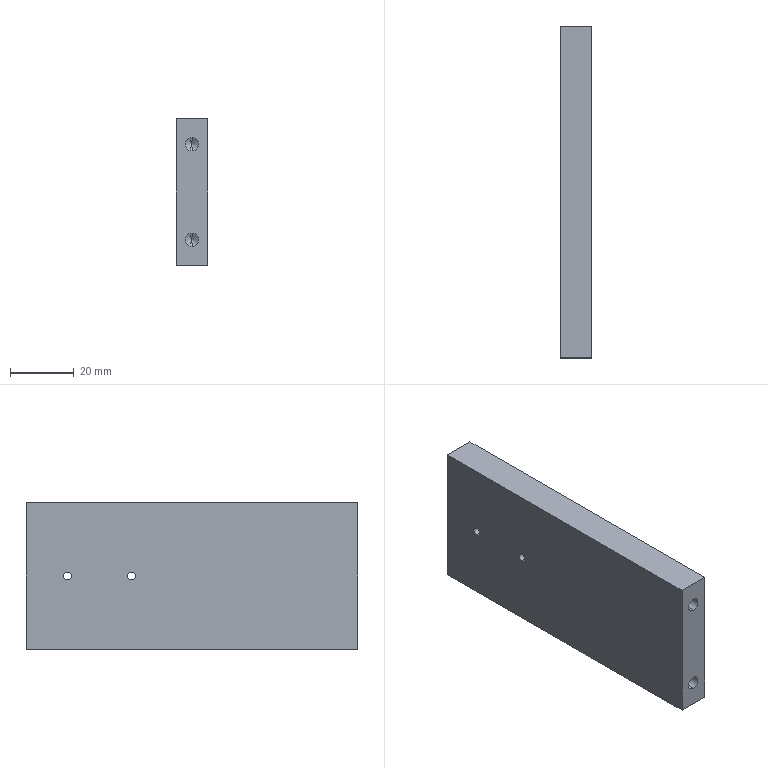Part | STEP file | 2058 Cylinder mounting plate | 1 solid | 18 faces | box 10 x 104 x 46 mm | volume 47342 mm3 | cylinder 8 | plane 6 | cone 4 | commonest cylinder face diameters 2.5 x4 4.2 x4
STEP:
#1=CARTESIAN_POINT('',(0.,0.,0.));
#2=DIRECTION('',(0.,0.,1.));
#3=DIRECTION('',(1.,0.,0.));
#4=AXIS2_PLACEMENT_3D('',#1,#2,#3);
#5=CARTESIAN_POINT('',(0.,-38.,5.9));
#6=VERTEX_POINT('',#5);
#7=CARTESIAN_POINT('',(0.,-52.,5.9));
#8=VERTEX_POINT('',#7);
#9=CARTESIAN_POINT('',(0.,-52.,5.9));
#10=DIRECTION('',(0.,-1.,0.));
#11=VECTOR('',#10,1.);
#12=LINE('',#9,#11);
#13=CARTESIAN_POINT('',(0.,-52.,8.));
#14=DIRECTION('',(0.,-1.,0.));
#15=DIRECTION('',(0.,0.,-1.));
#16=AXIS2_PLACEMENT_3D('',#13,#14,#15);
#17=CYLINDRICAL_SURFACE('',#16,2.1);
#18=CARTESIAN_POINT('',(6.283,0.));
#19=DIRECTION('',(0.,1.));
#20=VECTOR('',#19,1.);
#21=LINE('',#18,#20);
#22=(GEOMETRIC_REPRESENTATION_CONTEXT(2)PARAMETRIC_REPRESENTATION_CONTEXT()REPRESENTATION_CONTEXT('',''));
#23=DEFINITIONAL_REPRESENTATION('',(#21),#22);
#24=PCURVE('',#17,#23);
#25=CARTESIAN_POINT('',(0.,-52.,8.));
#26=DIRECTION('',(0.,-1.,0.));
#27=DIRECTION('',(0.,0.,-1.));
#28=AXIS2_PLACEMENT_3D('',#25,#26,#27);
#29=CYLINDRICAL_SURFACE('',#28,2.1);
#30=CARTESIAN_POINT('',(0.,0.));
#31=DIRECTION('',(0.,1.));
#32=VECTOR('',#31,1.);
#33=LINE('',#30,#32);
#34=(GEOMETRIC_REPRESENTATION_CONTEXT(2)PARAMETRIC_REPRESENTATION_CONTEXT()REPRESENTATION_CONTEXT('',''));
#35=DEFINITIONAL_REPRESENTATION('',(#33),#34);
#36=PCURVE('',#29,#35);
#37=SURFACE_CURVE('',#12,(#24,#36),.PCURVE_S1.);
#38=EDGE_CURVE('',#6,#8,#37,.T.);
#39=ORIENTED_EDGE('',*,*,#38,.T.);
#40=CARTESIAN_POINT('',(0.,-52.,10.1));
#41=VERTEX_POINT('',#40);
#42=CARTESIAN_POINT('',(0.,-52.,8.));
#43=DIRECTION('',(0.,-1.,0.));
#44=DIRECTION('',(0.,0.,-1.));
#45=AXIS2_PLACEMENT_3D('',#42,#43,#44);
#46=CIRCLE('',#45,2.1);
#47=CARTESIAN_POINT('',(0.,0.));
#48=DIRECTION('',(1.,0.));
#49=VECTOR('',#48,1.);
#50=LINE('',#47,#49);
#51=(GEOMETRIC_REPRESENTATION_CONTEXT(2)PARAMETRIC_REPRESENTATION_CONTEXT()REPRESENTATION_CONTEXT('',''));
#52=DEFINITIONAL_REPRESENTATION('',(#50),#51);
#53=PCURVE('',#17,#52);
#54=CARTESIAN_POINT('',(-5.,-52.,46.));
#55=DIRECTION('',(0.,1.,0.));
#56=DIRECTION('',(0.,0.,1.));
#57=AXIS2_PLACEMENT_3D('',#54,#55,#56);
#58=PLANE('',#57);
#59=CARTESIAN_POINT('',(-40.1,5.));
#60=CARTESIAN_POINT('',(-40.1,8.637));
#61=CARTESIAN_POINT('',(-36.95,6.819));
#62=CARTESIAN_POINT('',(-33.8,5.));
#63=CARTESIAN_POINT('',(-36.95,3.181));
#64=CARTESIAN_POINT('',(-40.1,1.363));
#65=CARTESIAN_POINT('',(-40.1,5.));
#66=(BOUNDED_CURVE()B_SPLINE_CURVE(2,(#59,#60,#61,#62,#63,#64,#65),.UNSPECIFIED.,.T.,.F.)B_SPLINE_CURVE_WITH_KNOTS((1,2,2,2,2,1),(-2.094,0.,2.094,4.189,6.283,8.378),.UNSPECIFIED.)CURVE()GEOMETRIC_REPRESENTATION_ITEM()RATIONAL_B_SPLINE_CURVE((1.,0.5,1.,0.5,1.,0.5,1.))REPRESENTATION_ITEM(''));
#67=(GEOMETRIC_REPRESENTATION_CONTEXT(2)PARAMETRIC_REPRESENTATION_CONTEXT()REPRESENTATION_CONTEXT('',''));
#68=DEFINITIONAL_REPRESENTATION('',(#66),#67);
#69=PCURVE('',#58,#68);
#70=SURFACE_CURVE('',#46,(#53,#69),.PCURVE_S1.);
#71=EDGE_CURVE('',#41,#8,#70,.T.);
#72=ORIENTED_EDGE('',*,*,#71,.F.);
#73=CARTESIAN_POINT('',(0.,-38.,10.1));
#74=VERTEX_POINT('',#73);
#75=CARTESIAN_POINT('',(0.,-52.,10.1));
#76=DIRECTION('',(0.,-1.,0.));
#77=VECTOR('',#76,1.);
#78=LINE('',#75,#77);
#79=CARTESIAN_POINT('',(3.142,0.));
#80=DIRECTION('',(0.,1.));
#81=VECTOR('',#80,1.);
#82=LINE('',#79,#81);
#83=(GEOMETRIC_REPRESENTATION_CONTEXT(2)PARAMETRIC_REPRESENTATION_CONTEXT()REPRESENTATION_CONTEXT('',''));
#84=DEFINITIONAL_REPRESENTATION('',(#82),#83);
#85=PCURVE('',#17,#84);
#86=CARTESIAN_POINT('',(3.142,0.));
#87=DIRECTION('',(0.,1.));
#88=VECTOR('',#87,1.);
#89=LINE('',#86,#88);
#90=(GEOMETRIC_REPRESENTATION_CONTEXT(2)PARAMETRIC_REPRESENTATION_CONTEXT()REPRESENTATION_CONTEXT('',''));
#91=DEFINITIONAL_REPRESENTATION('',(#89),#90);
#92=PCURVE('',#29,#91);
#93=SURFACE_CURVE('',#78,(#85,#92),.PCURVE_S1.);
#94=EDGE_CURVE('',#74,#41,#93,.T.);
#95=ORIENTED_EDGE('',*,*,#94,.F.);
#96=CARTESIAN_POINT('',(0.,-38.,8.));
#97=DIRECTION('',(0.,-1.,0.));
#98=DIRECTION('',(0.,0.,-1.));
#99=AXIS2_PLACEMENT_3D('',#96,#97,#98);
#100=CIRCLE('',#99,2.1);
#101=CARTESIAN_POINT('',(0.,-14.));
#102=DIRECTION('',(1.,0.));
#103=VECTOR('',#102,1.);
#104=LINE('',#101,#103);
#105=(GEOMETRIC_REPRESENTATION_CONTEXT(2)PARAMETRIC_REPRESENTATION_CONTEXT()REPRESENTATION_CONTEXT('',''));
#106=DEFINITIONAL_REPRESENTATION('',(#104),#105);
#107=PCURVE('',#17,#106);
#108=CARTESIAN_POINT('',(0.,-38.,8.));
#109=DIRECTION('',(0.,-1.,0.));
#110=DIRECTION('',(0.,0.,-1.));
#111=AXIS2_PLACEMENT_3D('',#108,#109,#110);
#112=CONICAL_SURFACE('',#111,2.1,1.03);
#113=CARTESIAN_POINT('',(0.,0.));
#114=DIRECTION('',(1.,0.));
#115=VECTOR('',#114,1.);
#116=LINE('',#113,#115);
#117=(GEOMETRIC_REPRESENTATION_CONTEXT(2)PARAMETRIC_REPRESENTATION_CONTEXT()REPRESENTATION_CONTEXT('',''));
#118=DEFINITIONAL_REPRESENTATION('',(#116),#117);
#119=PCURVE('',#112,#118);
#120=SURFACE_CURVE('',#100,(#107,#119),.PCURVE_S1.);
#121=EDGE_CURVE('',#74,#6,#120,.T.);
#122=ORIENTED_EDGE('',*,*,#121,.T.);
#123=EDGE_LOOP('',(#39,#72,#95,#122));
#124=FACE_BOUND('',#123,.F.);
#125=ADVANCED_FACE('',(#124),#17,.F.);
#126=ORIENTED_EDGE('',*,*,#121,.F.);
#127=CARTESIAN_POINT('',(0.,-36.738,8.));
#128=VERTEX_POINT('',#127);
#129=CARTESIAN_POINT('',(0.,-38.,10.1));
#130=DIRECTION('',(0.,-0.515,0.8572));
#131=VECTOR('',#130,1.);
#132=LINE('',#129,#131);
#133=CARTESIAN_POINT('',(3.142,0.));
#134=DIRECTION('',(0.,1.));
#135=VECTOR('',#134,1.);
#136=LINE('',#133,#135);
#137=(GEOMETRIC_REPRESENTATION_CONTEXT(2)PARAMETRIC_REPRESENTATION_CONTEXT()REPRESENTATION_CONTEXT('',''));
#138=DEFINITIONAL_REPRESENTATION('',(#136),#137);
#139=PCURVE('',#112,#138);
#140=CARTESIAN_POINT('',(0.,-38.,8.));
#141=DIRECTION('',(0.,-1.,0.));
#142=DIRECTION('',(0.,0.,-1.));
#143=AXIS2_PLACEMENT_3D('',#140,#141,#142);
#144=CONICAL_SURFACE('',#143,2.1,1.03);
#145=CARTESIAN_POINT('',(3.142,0.));
#146=DIRECTION('',(0.,1.));
#147=VECTOR('',#146,1.);
#148=LINE('',#145,#147);
#149=(GEOMETRIC_REPRESENTATION_CONTEXT(2)PARAMETRIC_REPRESENTATION_CONTEXT()REPRESENTATION_CONTEXT('',''));
#150=DEFINITIONAL_REPRESENTATION('',(#148),#149);
#151=PCURVE('',#144,#150);
#152=SURFACE_CURVE('',#132,(#139,#151),.PCURVE_S1.);
#153=EDGE_CURVE('',#128,#74,#152,.T.);
#154=ORIENTED_EDGE('',*,*,#153,.F.);
#155=CARTESIAN_POINT('',(0.,-38.,5.9));
#156=DIRECTION('',(0.,-0.515,-0.8572));
#157=VECTOR('',#156,1.);
#158=LINE('',#155,#157);
#159=CARTESIAN_POINT('',(6.283,0.));
#160=DIRECTION('',(0.,1.));
#161=VECTOR('',#160,1.);
#162=LINE('',#159,#161);
#163=(GEOMETRIC_REPRESENTATION_CONTEXT(2)PARAMETRIC_REPRESENTATION_CONTEXT()REPRESENTATION_CONTEXT('',''));
#164=DEFINITIONAL_REPRESENTATION('',(#162),#163);
#165=PCURVE('',#112,#164);
#166=CARTESIAN_POINT('',(0.,0.));
#167=DIRECTION('',(0.,1.));
#168=VECTOR('',#167,1.);
#169=LINE('',#166,#168);
#170=(GEOMETRIC_REPRESENTATION_CONTEXT(2)PARAMETRIC_REPRESENTATION_CONTEXT()REPRESENTATION_CONTEXT('',''));
#171=DEFINITIONAL_REPRESENTATION('',(#169),#170);
#172=PCURVE('',#144,#171);
#173=SURFACE_CURVE('',#158,(#165,#172),.PCURVE_S1.);
#174=EDGE_CURVE('',#128,#6,#173,.T.);
#175=ORIENTED_EDGE('',*,*,#174,.T.);
#176=EDGE_LOOP('',(#126,#154,#175));
#177=FACE_BOUND('',#176,.F.);
#178=ADVANCED_FACE('',(#177),#112,.F.);
#179=CARTESIAN_POINT('',(0.,-38.,35.9));
#180=VERTEX_POINT('',#179);
#181=CARTESIAN_POINT('',(0.,-52.,35.9));
#182=VERTEX_POINT('',#181);
#183=CARTESIAN_POINT('',(0.,-52.,35.9));
#184=DIRECTION('',(0.,-1.,0.));
#185=VECTOR('',#184,1.);
#186=LINE('',#183,#185);
#187=CARTESIAN_POINT('',(0.,-52.,38.));
#188=DIRECTION('',(0.,-1.,0.));
#189=DIRECTION('',(0.,0.,-1.));
#190=AXIS2_PLACEMENT_3D('',#187,#188,#189);
#191=CYLINDRICAL_SURFACE('',#190,2.1);
#192=CARTESIAN_POINT('',(6.283,0.));
#193=DIRECTION('',(0.,1.));
#194=VECTOR('',#193,1.);
#195=LINE('',#192,#194);
#196=(GEOMETRIC_REPRESENTATION_CONTEXT(2)PARAMETRIC_REPRESENTATION_CONTEXT()REPRESENTATION_CONTEXT('',''));
#197=DEFINITIONAL_REPRESENTATION('',(#195),#196);
#198=PCURVE('',#191,#197);
#199=CARTESIAN_POINT('',(0.,-52.,38.));
#200=DIRECTION('',(0.,-1.,0.));
#201=DIRECTION('',(0.,0.,-1.));
#202=AXIS2_PLACEMENT_3D('',#199,#200,#201);
#203=CYLINDRICAL_SURFACE('',#202,2.1);
#204=CARTESIAN_POINT('',(0.,0.));
#205=DIRECTION('',(0.,1.));
#206=VECTOR('',#205,1.);
#207=LINE('',#204,#206);
#208=(GEOMETRIC_REPRESENTATION_CONTEXT(2)PARAMETRIC_REPRESENTATION_CONTEXT()REPRESENTATION_CONTEXT('',''));
#209=DEFINITIONAL_REPRESENTATION('',(#207),#208);
#210=PCURVE('',#203,#209);
#211=SURFACE_CURVE('',#186,(#198,#210),.PCURVE_S1.);
#212=EDGE_CURVE('',#180,#182,#211,.T.);
#213=ORIENTED_EDGE('',*,*,#212,.T.);
#214=CARTESIAN_POINT('',(0.,-52.,40.1));
#215=VERTEX_POINT('',#214);
#216=CARTESIAN_POINT('',(0.,-52.,38.));
#217=DIRECTION('',(0.,-1.,0.));
#218=DIRECTION('',(0.,0.,-1.));
#219=AXIS2_PLACEMENT_3D('',#216,#217,#218);
#220=CIRCLE('',#219,2.1);
#221=CARTESIAN_POINT('',(0.,0.));
#222=DIRECTION('',(1.,0.));
#223=VECTOR('',#222,1.);
#224=LINE('',#221,#223);
#225=(GEOMETRIC_REPRESENTATION_CONTEXT(2)PARAMETRIC_REPRESENTATION_CONTEXT()REPRESENTATION_CONTEXT('',''));
#226=DEFINITIONAL_REPRESENTATION('',(#224),#225);
#227=PCURVE('',#191,#226);
#228=CARTESIAN_POINT('',(-10.1,5.));
#229=CARTESIAN_POINT('',(-10.1,8.637));
#230=CARTESIAN_POINT('',(-6.95,6.819));
#231=CARTESIAN_POINT('',(-3.8,5.));
#232=CARTESIAN_POINT('',(-6.95,3.181));
#233=CARTESIAN_POINT('',(-10.1,1.363));
#234=CARTESIAN_POINT('',(-10.1,5.));
#235=(BOUNDED_CURVE()B_SPLINE_CURVE(2,(#228,#229,#230,#231,#232,#233,#234),.UNSPECIFIED.,.T.,.F.)B_SPLINE_CURVE_WITH_KNOTS((1,2,2,2,2,1),(-2.094,0.,2.094,4.189,6.283,8.378),.UNSPECIFIED.)CURVE()GEOMETRIC_REPRESENTATION_ITEM()RATIONAL_B_SPLINE_CURVE((1.,0.5,1.,0.5,1.,0.5,1.))REPRESENTATION_ITEM(''));
#236=(GEOMETRIC_REPRESENTATION_CONTEXT(2)PARAMETRIC_REPRESENTATION_CONTEXT()REPRESENTATION_CONTEXT('',''));
#237=DEFINITIONAL_REPRESENTATION('',(#235),#236);
#238=PCURVE('',#58,#237);
#239=SURFACE_CURVE('',#220,(#227,#238),.PCURVE_S1.);
#240=EDGE_CURVE('',#215,#182,#239,.T.);
#241=ORIENTED_EDGE('',*,*,#240,.F.);
#242=CARTESIAN_POINT('',(0.,-38.,40.1));
#243=VERTEX_POINT('',#242);
#244=CARTESIAN_POINT('',(0.,-52.,40.1));
#245=DIRECTION('',(0.,-1.,0.));
#246=VECTOR('',#245,1.);
#247=LINE('',#244,#246);
#248=CARTESIAN_POINT('',(3.142,0.));
#249=DIRECTION('',(0.,1.));
#250=VECTOR('',#249,1.);
#251=LINE('',#248,#250);
#252=(GEOMETRIC_REPRESENTATION_CONTEXT(2)PARAMETRIC_REPRESENTATION_CONTEXT()REPRESENTATION_CONTEXT('',''));
#253=DEFINITIONAL_REPRESENTATION('',(#251),#252);
#254=PCURVE('',#191,#253);
#255=CARTESIAN_POINT('',(3.142,0.));
#256=DIRECTION('',(0.,1.));
#257=VECTOR('',#256,1.);
#258=LINE('',#255,#257);
#259=(GEOMETRIC_REPRESENTATION_CONTEXT(2)PARAMETRIC_REPRESENTATION_CONTEXT()REPRESENTATION_CONTEXT('',''));
#260=DEFINITIONAL_REPRESENTATION('',(#258),#259);
#261=PCURVE('',#203,#260);
#262=SURFACE_CURVE('',#247,(#254,#261),.PCURVE_S1.);
#263=EDGE_CURVE('',#243,#215,#262,.T.);
#264=ORIENTED_EDGE('',*,*,#263,.F.);
#265=CARTESIAN_POINT('',(0.,-38.,38.));
#266=DIRECTION('',(0.,-1.,0.));
#267=DIRECTION('',(0.,0.,-1.));
#268=AXIS2_PLACEMENT_3D('',#265,#266,#267);
#269=CIRCLE('',#268,2.1);
#270=CARTESIAN_POINT('',(0.,-14.));
#271=DIRECTION('',(1.,0.));
#272=VECTOR('',#271,1.);
#273=LINE('',#270,#272);
#274=(GEOMETRIC_REPRESENTATION_CONTEXT(2)PARAMETRIC_REPRESENTATION_CONTEXT()REPRESENTATION_CONTEXT('',''));
#275=DEFINITIONAL_REPRESENTATION('',(#273),#274);
#276=PCURVE('',#191,#275);
#277=CARTESIAN_POINT('',(0.,-38.,38.));
#278=DIRECTION('',(0.,-1.,0.));
#279=DIRECTION('',(0.,0.,-1.));
#280=AXIS2_PLACEMENT_3D('',#277,#278,#279);
#281=CONICAL_SURFACE('',#280,2.1,1.03);
#282=CARTESIAN_POINT('',(0.,0.));
#283=DIRECTION('',(1.,0.));
#284=VECTOR('',#283,1.);
#285=LINE('',#282,#284);
#286=(GEOMETRIC_REPRESENTATION_CONTEXT(2)PARAMETRIC_REPRESENTATION_CONTEXT()REPRESENTATION_CONTEXT('',''));
#287=DEFINITIONAL_REPRESENTATION('',(#285),#286);
#288=PCURVE('',#281,#287);
#289=SURFACE_CURVE('',#269,(#276,#288),.PCURVE_S1.);
#290=EDGE_CURVE('',#243,#180,#289,.T.);
#291=ORIENTED_EDGE('',*,*,#290,.T.);
#292=EDGE_LOOP('',(#213,#241,#264,#291));
#293=FACE_BOUND('',#292,.F.);
#294=ADVANCED_FACE('',(#293),#191,.F.);
#295=ORIENTED_EDGE('',*,*,#290,.F.);
#296=CARTESIAN_POINT('',(0.,-36.738,38.));
#297=VERTEX_POINT('',#296);
#298=CARTESIAN_POINT('',(0.,-38.,40.1));
#299=DIRECTION('',(0.,-0.515,0.8572));
#300=VECTOR('',#299,1.);
#301=LINE('',#298,#300);
#302=CARTESIAN_POINT('',(3.142,-1.262));
#303=CARTESIAN_POINT('',(3.142,-1.243));
#304=CARTESIAN_POINT('',(3.142,-1.204));
#305=CARTESIAN_POINT('',(3.142,-1.147));
#306=CARTESIAN_POINT('',(3.142,-1.09));
#307=CARTESIAN_POINT('',(3.142,-1.032));
#308=CARTESIAN_POINT('',(3.142,-0.975));
#309=CARTESIAN_POINT('',(3.142,-0.9177));
#310=CARTESIAN_POINT('',(3.142,-0.8603));
#311=CARTESIAN_POINT('',(3.142,-0.803));
#312=CARTESIAN_POINT('',(3.142,-0.7456));
#313=CARTESIAN_POINT('',(3.142,-0.6883));
#314=CARTESIAN_POINT('',(3.142,-0.6309));
#315=CARTESIAN_POINT('',(3.142,-0.5735));
#316=CARTESIAN_POINT('',(3.142,-0.5162));
#317=CARTESIAN_POINT('',(3.142,-0.4588));
#318=CARTESIAN_POINT('',(3.142,-0.4015));
#319=CARTESIAN_POINT('',(3.142,-0.3441));
#320=CARTESIAN_POINT('',(3.142,-0.2868));
#321=CARTESIAN_POINT('',(3.142,-0.2294));
#322=CARTESIAN_POINT('',(3.142,-0.1721));
#323=CARTESIAN_POINT('',(3.142,-0.1147));
#324=CARTESIAN_POINT('',(3.142,-0.05735));
#325=CARTESIAN_POINT('',(3.142,-0.01912));
#326=CARTESIAN_POINT('',(3.142,0.));
#327=B_SPLINE_CURVE_WITH_KNOTS('',3,(#302,#303,#304,#305,#306,#307,#308,#309,#310,#311,#312,#313,#314,#315,#316,#317,#318,#319,#320,#321,#322,#323,#324,#325,#326),.UNSPECIFIED.,.F.,.F.,(4,1,1,1,1,1,1,1,1,1,1,1,1,1,1,1,1,1,1,1,1,1,4),(-2.45,-2.339,-2.227,-2.116,-2.004,-1.893,-1.782,-1.67,-1.559,-1.448,-1.336,-1.225,-1.114,-1.002,-0.8909,-0.7795,-0.6682,-0.5568,-0.4454,-0.3341,-0.2227,-0.1114,0.),.QUASI_UNIFORM_KNOTS.);
#328=(GEOMETRIC_REPRESENTATION_CONTEXT(2)PARAMETRIC_REPRESENTATION_CONTEXT()REPRESENTATION_CONTEXT('',''));
#329=DEFINITIONAL_REPRESENTATION('',(#327),#328);
#330=PCURVE('',#281,#329);
#331=CARTESIAN_POINT('',(0.,-38.,38.));
#332=DIRECTION('',(0.,-1.,0.));
#333=DIRECTION('',(0.,0.,-1.));
#334=AXIS2_PLACEMENT_3D('',#331,#332,#333);
#335=CONICAL_SURFACE('',#334,2.1,1.03);
#336=CARTESIAN_POINT('',(3.142,-1.262));
#337=CARTESIAN_POINT('',(3.142,-1.243));
#338=CARTESIAN_POINT('',(3.142,-1.204));
#339=CARTESIAN_POINT('',(3.142,-1.147));
#340=CARTESIAN_POINT('',(3.142,-1.09));
#341=CARTESIAN_POINT('',(3.142,-1.032));
#342=CARTESIAN_POINT('',(3.142,-0.975));
#343=CARTESIAN_POINT('',(3.142,-0.9177));
#344=CARTESIAN_POINT('',(3.142,-0.8603));
#345=CARTESIAN_POINT('',(3.142,-0.803));
#346=CARTESIAN_POINT('',(3.142,-0.7456));
#347=CARTESIAN_POINT('',(3.142,-0.6883));
#348=CARTESIAN_POINT('',(3.142,-0.6309));
#349=CARTESIAN_POINT('',(3.142,-0.5735));
#350=CARTESIAN_POINT('',(3.142,-0.5162));
#351=CARTESIAN_POINT('',(3.142,-0.4588));
#352=CARTESIAN_POINT('',(3.142,-0.4015));
#353=CARTESIAN_POINT('',(3.142,-0.3441));
#354=CARTESIAN_POINT('',(3.142,-0.2868));
#355=CARTESIAN_POINT('',(3.142,-0.2294));
#356=CARTESIAN_POINT('',(3.142,-0.1721));
#357=CARTESIAN_POINT('',(3.142,-0.1147));
#358=CARTESIAN_POINT('',(3.142,-0.05735));
#359=CARTESIAN_POINT('',(3.142,-0.01912));
#360=CARTESIAN_POINT('',(3.142,0.));
#361=B_SPLINE_CURVE_WITH_KNOTS('',3,(#336,#337,#338,#339,#340,#341,#342,#343,#344,#345,#346,#347,#348,#349,#350,#351,#352,#353,#354,#355,#356,#357,#358,#359,#360),.UNSPECIFIED.,.F.,.F.,(4,1,1,1,1,1,1,1,1,1,1,1,1,1,1,1,1,1,1,1,1,1,4),(-2.45,-2.339,-2.227,-2.116,-2.004,-1.893,-1.782,-1.67,-1.559,-1.448,-1.336,-1.225,-1.114,-1.002,-0.8909,-0.7795,-0.6682,-0.5568,-0.4454,-0.3341,-0.2227,-0.1114,0.),.QUASI_UNIFORM_KNOTS.);
#362=(GEOMETRIC_REPRESENTATION_CONTEXT(2)PARAMETRIC_REPRESENTATION_CONTEXT()REPRESENTATION_CONTEXT('',''));
#363=DEFINITIONAL_REPRESENTATION('',(#361),#362);
#364=PCURVE('',#335,#363);
#365=SURFACE_CURVE('',#301,(#330,#364),.PCURVE_S1.);
#366=EDGE_CURVE('',#297,#243,#365,.T.);
#367=ORIENTED_EDGE('',*,*,#366,.F.);
#368=CARTESIAN_POINT('',(0.,-38.,35.9));
#369=DIRECTION('',(0.,-0.515,-0.8572));
#370=VECTOR('',#369,1.);
#371=LINE('',#368,#370);
#372=CARTESIAN_POINT('',(6.283,0.));
#373=DIRECTION('',(0.,1.));
#374=VECTOR('',#373,1.);
#375=LINE('',#372,#374);
#376=(GEOMETRIC_REPRESENTATION_CONTEXT(2)PARAMETRIC_REPRESENTATION_CONTEXT()REPRESENTATION_CONTEXT('',''));
#377=DEFINITIONAL_REPRESENTATION('',(#375),#376);
#378=PCURVE('',#281,#377);
#379=CARTESIAN_POINT('',(0.,0.));
#380=DIRECTION('',(0.,1.));
#381=VECTOR('',#380,1.);
#382=LINE('',#379,#381);
#383=(GEOMETRIC_REPRESENTATION_CONTEXT(2)PARAMETRIC_REPRESENTATION_CONTEXT()REPRESENTATION_CONTEXT('',''));
#384=DEFINITIONAL_REPRESENTATION('',(#382),#383);
#385=PCURVE('',#335,#384);
#386=SURFACE_CURVE('',#371,(#378,#385),.PCURVE_S1.);
#387=EDGE_CURVE('',#297,#180,#386,.T.);
#388=ORIENTED_EDGE('',*,*,#387,.T.);
#389=EDGE_LOOP('',(#295,#367,#388));
#390=FACE_BOUND('',#389,.F.);
#391=ADVANCED_FACE('',(#390),#281,.F.);
#392=CARTESIAN_POINT('',(-5.,19.,21.75));
#393=VERTEX_POINT('',#392);
#394=CARTESIAN_POINT('',(5.,19.,21.75));
#395=VERTEX_POINT('',#394);
#396=CARTESIAN_POINT('',(5.,19.,21.75));
#397=DIRECTION('',(1.,0.,0.));
#398=VECTOR('',#397,1.);
#399=LINE('',#396,#398);
#400=CARTESIAN_POINT('',(5.,19.,23.));
#401=DIRECTION('',(1.,0.,0.));
#402=DIRECTION('',(0.,0.,-1.));
#403=AXIS2_PLACEMENT_3D('',#400,#401,#402);
#404=CYLINDRICAL_SURFACE('',#403,1.25);
#405=CARTESIAN_POINT('',(6.283,0.));
#406=DIRECTION('',(0.,1.));
#407=VECTOR('',#406,1.);
#408=LINE('',#405,#407);
#409=(GEOMETRIC_REPRESENTATION_CONTEXT(2)PARAMETRIC_REPRESENTATION_CONTEXT()REPRESENTATION_CONTEXT('',''));
#410=DEFINITIONAL_REPRESENTATION('',(#408),#409);
#411=PCURVE('',#404,#410);
#412=CARTESIAN_POINT('',(5.,19.,23.));
#413=DIRECTION('',(1.,0.,0.));
#414=DIRECTION('',(0.,0.,-1.));
#415=AXIS2_PLACEMENT_3D('',#412,#413,#414);
#416=CYLINDRICAL_SURFACE('',#415,1.25);
#417=CARTESIAN_POINT('',(0.,0.));
#418=DIRECTION('',(0.,1.));
#419=VECTOR('',#418,1.);
#420=LINE('',#417,#419);
#421=(GEOMETRIC_REPRESENTATION_CONTEXT(2)PARAMETRIC_REPRESENTATION_CONTEXT()REPRESENTATION_CONTEXT('',''));
#422=DEFINITIONAL_REPRESENTATION('',(#420),#421);
#423=PCURVE('',#416,#422);
#424=SURFACE_CURVE('',#399,(#411,#423),.PCURVE_S1.);
#425=EDGE_CURVE('',#393,#395,#424,.T.);
#426=ORIENTED_EDGE('',*,*,#425,.T.);
#427=CARTESIAN_POINT('',(5.,19.,24.25));
#428=VERTEX_POINT('',#427);
#429=CARTESIAN_POINT('',(5.,19.,23.));
#430=DIRECTION('',(1.,0.,0.));
#431=DIRECTION('',(0.,0.,-1.));
#432=AXIS2_PLACEMENT_3D('',#429,#430,#431);
#433=CIRCLE('',#432,1.25);
#434=CARTESIAN_POINT('',(0.,0.));
#435=DIRECTION('',(1.,0.));
#436=VECTOR('',#435,1.);
#437=LINE('',#434,#436);
#438=(GEOMETRIC_REPRESENTATION_CONTEXT(2)PARAMETRIC_REPRESENTATION_CONTEXT()REPRESENTATION_CONTEXT('',''));
#439=DEFINITIONAL_REPRESENTATION('',(#437),#438);
#440=PCURVE('',#404,#439);
#441=CARTESIAN_POINT('',(5.,-52.,46.));
#442=DIRECTION('',(-1.,0.,0.));
#443=DIRECTION('',(0.,0.,1.));
#444=AXIS2_PLACEMENT_3D('',#441,#442,#443);
#445=PLANE('',#444);
#446=CARTESIAN_POINT('',(-24.25,71.));
#447=CARTESIAN_POINT('',(-24.25,73.165));
#448=CARTESIAN_POINT('',(-22.375,72.083));
#449=CARTESIAN_POINT('',(-20.5,71.));
#450=CARTESIAN_POINT('',(-22.375,69.917));
#451=CARTESIAN_POINT('',(-24.25,68.835));
#452=CARTESIAN_POINT('',(-24.25,71.));
#453=(BOUNDED_CURVE()B_SPLINE_CURVE(2,(#446,#447,#448,#449,#450,#451,#452),.UNSPECIFIED.,.T.,.F.)B_SPLINE_CURVE_WITH_KNOTS((1,2,2,2,2,1),(-2.094,0.,2.094,4.189,6.283,8.378),.UNSPECIFIED.)CURVE()GEOMETRIC_REPRESENTATION_ITEM()RATIONAL_B_SPLINE_CURVE((1.,0.5,1.,0.5,1.,0.5,1.))REPRESENTATION_ITEM(''));
#454=(GEOMETRIC_REPRESENTATION_CONTEXT(2)PARAMETRIC_REPRESENTATION_CONTEXT()REPRESENTATION_CONTEXT('',''));
#455=DEFINITIONAL_REPRESENTATION('',(#453),#454);
#456=PCURVE('',#445,#455);
#457=SURFACE_CURVE('',#433,(#440,#456),.PCURVE_S1.);
#458=EDGE_CURVE('',#428,#395,#457,.T.);
#459=ORIENTED_EDGE('',*,*,#458,.F.);
#460=CARTESIAN_POINT('',(-5.,19.,24.25));
#461=VERTEX_POINT('',#460);
#462=CARTESIAN_POINT('',(5.,19.,24.25));
#463=DIRECTION('',(1.,0.,0.));
#464=VECTOR('',#463,1.);
#465=LINE('',#462,#464);
#466=CARTESIAN_POINT('',(3.142,0.));
#467=DIRECTION('',(0.,1.));
#468=VECTOR('',#467,1.);
#469=LINE('',#466,#468);
#470=(GEOMETRIC_REPRESENTATION_CONTEXT(2)PARAMETRIC_REPRESENTATION_CONTEXT()REPRESENTATION_CONTEXT('',''));
#471=DEFINITIONAL_REPRESENTATION('',(#469),#470);
#472=PCURVE('',#404,#471);
#473=CARTESIAN_POINT('',(3.142,0.));
#474=DIRECTION('',(0.,1.));
#475=VECTOR('',#474,1.);
#476=LINE('',#473,#475);
#477=(GEOMETRIC_REPRESENTATION_CONTEXT(2)PARAMETRIC_REPRESENTATION_CONTEXT()REPRESENTATION_CONTEXT('',''));
#478=DEFINITIONAL_REPRESENTATION('',(#476),#477);
#479=PCURVE('',#416,#478);
#480=SURFACE_CURVE('',#465,(#472,#479),.PCURVE_S1.);
#481=EDGE_CURVE('',#461,#428,#480,.T.);
#482=ORIENTED_EDGE('',*,*,#481,.F.);
#483=CARTESIAN_POINT('',(-5.,19.,23.));
#484=DIRECTION('',(1.,0.,0.));
#485=DIRECTION('',(0.,0.,-1.));
#486=AXIS2_PLACEMENT_3D('',#483,#484,#485);
#487=CIRCLE('',#486,1.25);
#488=CARTESIAN_POINT('',(0.,-10.));
#489=DIRECTION('',(1.,0.));
#490=VECTOR('',#489,1.);
#491=LINE('',#488,#490);
#492=(GEOMETRIC_REPRESENTATION_CONTEXT(2)PARAMETRIC_REPRESENTATION_CONTEXT()REPRESENTATION_CONTEXT('',''));
#493=DEFINITIONAL_REPRESENTATION('',(#491),#492);
#494=PCURVE('',#404,#493);
#495=CARTESIAN_POINT('',(-5.,-52.,46.));
#496=DIRECTION('',(1.,0.,0.));
#497=DIRECTION('',(0.,0.,-1.));
#498=AXIS2_PLACEMENT_3D('',#495,#496,#497);
#499=PLANE('',#498);
#500=CARTESIAN_POINT('',(23.,71.));
#501=DIRECTION('',(1.,0.));
#502=AXIS2_PLACEMENT_2D('',#500,#501);
#503=CIRCLE('',#502,1.25);
#504=(GEOMETRIC_REPRESENTATION_CONTEXT(2)PARAMETRIC_REPRESENTATION_CONTEXT()REPRESENTATION_CONTEXT('',''));
#505=DEFINITIONAL_REPRESENTATION('',(#503),#504);
#506=PCURVE('',#499,#505);
#507=SURFACE_CURVE('',#487,(#494,#506),.PCURVE_S1.);
#508=EDGE_CURVE('',#461,#393,#507,.T.);
#509=ORIENTED_EDGE('',*,*,#508,.T.);
#510=EDGE_LOOP('',(#426,#459,#482,#509));
#511=FACE_BOUND('',#510,.F.);
#512=ADVANCED_FACE('',(#511),#404,.F.);
#513=CARTESIAN_POINT('',(-5.,39.,21.75));
#514=VERTEX_POINT('',#513);
#515=CARTESIAN_POINT('',(5.,39.,21.75));
#516=VERTEX_POINT('',#515);
#517=CARTESIAN_POINT('',(5.,39.,21.75));
#518=DIRECTION('',(1.,0.,0.));
#519=VECTOR('',#518,1.);
#520=LINE('',#517,#519);
#521=CARTESIAN_POINT('',(5.,39.,23.));
#522=DIRECTION('',(1.,0.,0.));
#523=DIRECTION('',(0.,0.,-1.));
#524=AXIS2_PLACEMENT_3D('',#521,#522,#523);
#525=CYLINDRICAL_SURFACE('',#524,1.25);
#526=CARTESIAN_POINT('',(6.283,0.));
#527=DIRECTION('',(0.,1.));
#528=VECTOR('',#527,1.);
#529=LINE('',#526,#528);
#530=(GEOMETRIC_REPRESENTATION_CONTEXT(2)PARAMETRIC_REPRESENTATION_CONTEXT()REPRESENTATION_CONTEXT('',''));
#531=DEFINITIONAL_REPRESENTATION('',(#529),#530);
#532=PCURVE('',#525,#531);
#533=CARTESIAN_POINT('',(5.,39.,23.));
#534=DIRECTION('',(1.,0.,0.));
#535=DIRECTION('',(0.,0.,-1.));
#536=AXIS2_PLACEMENT_3D('',#533,#534,#535);
#537=CYLINDRICAL_SURFACE('',#536,1.25);
#538=CARTESIAN_POINT('',(0.,0.));
#539=DIRECTION('',(0.,1.));
#540=VECTOR('',#539,1.);
#541=LINE('',#538,#540);
#542=(GEOMETRIC_REPRESENTATION_CONTEXT(2)PARAMETRIC_REPRESENTATION_CONTEXT()REPRESENTATION_CONTEXT('',''));
#543=DEFINITIONAL_REPRESENTATION('',(#541),#542);
#544=PCURVE('',#537,#543);
#545=SURFACE_CURVE('',#520,(#532,#544),.PCURVE_S1.);
#546=EDGE_CURVE('',#514,#516,#545,.T.);
#547=ORIENTED_EDGE('',*,*,#546,.T.);
#548=CARTESIAN_POINT('',(5.,39.,24.25));
#549=VERTEX_POINT('',#548);
#550=CARTESIAN_POINT('',(5.,39.,23.));
#551=DIRECTION('',(1.,0.,0.));
#552=DIRECTION('',(0.,0.,-1.));
#553=AXIS2_PLACEMENT_3D('',#550,#551,#552);
#554=CIRCLE('',#553,1.25);
#555=CARTESIAN_POINT('',(0.,0.));
#556=DIRECTION('',(1.,0.));
#557=VECTOR('',#556,1.);
#558=LINE('',#555,#557);
#559=(GEOMETRIC_REPRESENTATION_CONTEXT(2)PARAMETRIC_REPRESENTATION_CONTEXT()REPRESENTATION_CONTEXT('',''));
#560=DEFINITIONAL_REPRESENTATION('',(#558),#559);
#561=PCURVE('',#525,#560);
#562=CARTESIAN_POINT('',(-24.25,91.));
#563=CARTESIAN_POINT('',(-24.25,93.165));
#564=CARTESIAN_POINT('',(-22.375,92.083));
#565=CARTESIAN_POINT('',(-20.5,91.));
#566=CARTESIAN_POINT('',(-22.375,89.917));
#567=CARTESIAN_POINT('',(-24.25,88.835));
#568=CARTESIAN_POINT('',(-24.25,91.));
#569=(BOUNDED_CURVE()B_SPLINE_CURVE(2,(#562,#563,#564,#565,#566,#567,#568),.UNSPECIFIED.,.T.,.F.)B_SPLINE_CURVE_WITH_KNOTS((1,2,2,2,2,1),(-2.094,0.,2.094,4.189,6.283,8.378),.UNSPECIFIED.)CURVE()GEOMETRIC_REPRESENTATION_ITEM()RATIONAL_B_SPLINE_CURVE((1.,0.5,1.,0.5,1.,0.5,1.))REPRESENTATION_ITEM(''));
#570=(GEOMETRIC_REPRESENTATION_CONTEXT(2)PARAMETRIC_REPRESENTATION_CONTEXT()REPRESENTATION_CONTEXT('',''));
#571=DEFINITIONAL_REPRESENTATION('',(#569),#570);
#572=PCURVE('',#445,#571);
#573=SURFACE_CURVE('',#554,(#561,#572),.PCURVE_S1.);
#574=EDGE_CURVE('',#549,#516,#573,.T.);
#575=ORIENTED_EDGE('',*,*,#574,.F.);
#576=CARTESIAN_POINT('',(-5.,39.,24.25));
#577=VERTEX_POINT('',#576);
#578=CARTESIAN_POINT('',(5.,39.,24.25));
#579=DIRECTION('',(1.,0.,0.));
#580=VECTOR('',#579,1.);
#581=LINE('',#578,#580);
#582=CARTESIAN_POINT('',(3.142,0.));
#583=DIRECTION('',(0.,1.));
#584=VECTOR('',#583,1.);
#585=LINE('',#582,#584);
#586=(GEOMETRIC_REPRESENTATION_CONTEXT(2)PARAMETRIC_REPRESENTATION_CONTEXT()REPRESENTATION_CONTEXT('',''));
#587=DEFINITIONAL_REPRESENTATION('',(#585),#586);
#588=PCURVE('',#525,#587);
#589=CARTESIAN_POINT('',(3.142,0.));
#590=DIRECTION('',(0.,1.));
#591=VECTOR('',#590,1.);
#592=LINE('',#589,#591);
#593=(GEOMETRIC_REPRESENTATION_CONTEXT(2)PARAMETRIC_REPRESENTATION_CONTEXT()REPRESENTATION_CONTEXT('',''));
#594=DEFINITIONAL_REPRESENTATION('',(#592),#593);
#595=PCURVE('',#537,#594);
#596=SURFACE_CURVE('',#581,(#588,#595),.PCURVE_S1.);
#597=EDGE_CURVE('',#577,#549,#596,.T.);
#598=ORIENTED_EDGE('',*,*,#597,.F.);
#599=CARTESIAN_POINT('',(-5.,39.,23.));
#600=DIRECTION('',(1.,0.,0.));
#601=DIRECTION('',(0.,0.,-1.));
#602=AXIS2_PLACEMENT_3D('',#599,#600,#601);
#603=CIRCLE('',#602,1.25);
#604=CARTESIAN_POINT('',(0.,-10.));
#605=DIRECTION('',(1.,0.));
#606=VECTOR('',#605,1.);
#607=LINE('',#604,#606);
#608=(GEOMETRIC_REPRESENTATION_CONTEXT(2)PARAMETRIC_REPRESENTATION_CONTEXT()REPRESENTATION_CONTEXT('',''));
#609=DEFINITIONAL_REPRESENTATION('',(#607),#608);
#610=PCURVE('',#525,#609);
#611=CARTESIAN_POINT('',(23.,91.));
#612=DIRECTION('',(1.,0.));
#613=AXIS2_PLACEMENT_2D('',#611,#612);
#614=CIRCLE('',#613,1.25);
#615=(GEOMETRIC_REPRESENTATION_CONTEXT(2)PARAMETRIC_REPRESENTATION_CONTEXT()REPRESENTATION_CONTEXT('',''));
#616=DEFINITIONAL_REPRESENTATION('',(#614),#615);
#617=PCURVE('',#499,#616);
#618=SURFACE_CURVE('',#603,(#610,#617),.PCURVE_S1.);
#619=EDGE_CURVE('',#577,#514,#618,.T.);
#620=ORIENTED_EDGE('',*,*,#619,.T.);
#621=EDGE_LOOP('',(#547,#575,#598,#620));
#622=FACE_BOUND('',#621,.F.);
#623=ADVANCED_FACE('',(#622),#525,.F.);
#624=CARTESIAN_POINT('',(5.,19.,23.));
#625=DIRECTION('',(1.,0.,0.));
#626=DIRECTION('',(0.,0.,-1.));
#627=AXIS2_PLACEMENT_3D('',#624,#625,#626);
#628=CIRCLE('',#627,1.25);
#629=CARTESIAN_POINT('',(-24.25,71.));
#630=CARTESIAN_POINT('',(-24.25,73.165));
#631=CARTESIAN_POINT('',(-22.375,72.083));
#632=CARTESIAN_POINT('',(-20.5,71.));
#633=CARTESIAN_POINT('',(-22.375,69.917));
#634=CARTESIAN_POINT('',(-24.25,68.835));
#635=CARTESIAN_POINT('',(-24.25,71.));
#636=(BOUNDED_CURVE()B_SPLINE_CURVE(2,(#629,#630,#631,#632,#633,#634,#635),.UNSPECIFIED.,.T.,.F.)B_SPLINE_CURVE_WITH_KNOTS((1,2,2,2,2,1),(-2.094,0.,2.094,4.189,6.283,8.378),.UNSPECIFIED.)CURVE()GEOMETRIC_REPRESENTATION_ITEM()RATIONAL_B_SPLINE_CURVE((1.,0.5,1.,0.5,1.,0.5,1.))REPRESENTATION_ITEM(''));
#637=(GEOMETRIC_REPRESENTATION_CONTEXT(2)PARAMETRIC_REPRESENTATION_CONTEXT()REPRESENTATION_CONTEXT('',''));
#638=DEFINITIONAL_REPRESENTATION('',(#636),#637);
#639=PCURVE('',#445,#638);
#640=CARTESIAN_POINT('',(0.,0.));
#641=DIRECTION('',(1.,0.));
#642=VECTOR('',#641,1.);
#643=LINE('',#640,#642);
#644=(GEOMETRIC_REPRESENTATION_CONTEXT(2)PARAMETRIC_REPRESENTATION_CONTEXT()REPRESENTATION_CONTEXT('',''));
#645=DEFINITIONAL_REPRESENTATION('',(#643),#644);
#646=PCURVE('',#416,#645);
#647=SURFACE_CURVE('',#628,(#639,#646),.PCURVE_S1.);
#648=EDGE_CURVE('',#395,#428,#647,.T.);
#649=ORIENTED_EDGE('',*,*,#648,.F.);
#650=ORIENTED_EDGE('',*,*,#458,.F.);
#651=EDGE_LOOP('',(#649,#650));
#652=FACE_BOUND('',#651,.T.);
#653=CARTESIAN_POINT('',(5.,39.,23.));
#654=DIRECTION('',(1.,0.,0.));
#655=DIRECTION('',(0.,0.,-1.));
#656=AXIS2_PLACEMENT_3D('',#653,#654,#655);
#657=CIRCLE('',#656,1.25);
#658=CARTESIAN_POINT('',(-24.25,91.));
#659=CARTESIAN_POINT('',(-24.25,93.165));
#660=CARTESIAN_POINT('',(-22.375,92.083));
#661=CARTESIAN_POINT('',(-20.5,91.));
#662=CARTESIAN_POINT('',(-22.375,89.917));
#663=CARTESIAN_POINT('',(-24.25,88.835));
#664=CARTESIAN_POINT('',(-24.25,91.));
#665=(BOUNDED_CURVE()B_SPLINE_CURVE(2,(#658,#659,#660,#661,#662,#663,#664),.UNSPECIFIED.,.T.,.F.)B_SPLINE_CURVE_WITH_KNOTS((1,2,2,2,2,1),(-2.094,0.,2.094,4.189,6.283,8.378),.UNSPECIFIED.)CURVE()GEOMETRIC_REPRESENTATION_ITEM()RATIONAL_B_SPLINE_CURVE((1.,0.5,1.,0.5,1.,0.5,1.))REPRESENTATION_ITEM(''));
#666=(GEOMETRIC_REPRESENTATION_CONTEXT(2)PARAMETRIC_REPRESENTATION_CONTEXT()REPRESENTATION_CONTEXT('',''));
#667=DEFINITIONAL_REPRESENTATION('',(#665),#666);
#668=PCURVE('',#445,#667);
#669=CARTESIAN_POINT('',(0.,0.));
#670=DIRECTION('',(1.,0.));
#671=VECTOR('',#670,1.);
#672=LINE('',#669,#671);
#673=(GEOMETRIC_REPRESENTATION_CONTEXT(2)PARAMETRIC_REPRESENTATION_CONTEXT()REPRESENTATION_CONTEXT('',''));
#674=DEFINITIONAL_REPRESENTATION('',(#672),#673);
#675=PCURVE('',#537,#674);
#676=SURFACE_CURVE('',#657,(#668,#675),.PCURVE_S1.);
#677=EDGE_CURVE('',#516,#549,#676,.T.);
#678=ORIENTED_EDGE('',*,*,#677,.F.);
#679=ORIENTED_EDGE('',*,*,#574,.F.);
#680=EDGE_LOOP('',(#678,#679));
#681=FACE_BOUND('',#680,.T.);
#682=CARTESIAN_POINT('',(5.,-52.,0.));
#683=VERTEX_POINT('',#682);
#684=CARTESIAN_POINT('',(5.,52.,0.));
#685=VERTEX_POINT('',#684);
#686=CARTESIAN_POINT('',(5.,-52.,0.));
#687=DIRECTION('',(0.,1.,0.));
#688=VECTOR('',#687,1.);
#689=LINE('',#686,#688);
#690=CARTESIAN_POINT('',(-46.,0.));
#691=DIRECTION('',(0.,1.));
#692=VECTOR('',#691,1.);
#693=LINE('',#690,#692);
#694=(GEOMETRIC_REPRESENTATION_CONTEXT(2)PARAMETRIC_REPRESENTATION_CONTEXT()REPRESENTATION_CONTEXT('',''));
#695=DEFINITIONAL_REPRESENTATION('',(#693),#694);
#696=PCURVE('',#445,#695);
#697=CARTESIAN_POINT('',(0.,0.,0.));
#698=DIRECTION('',(0.,0.,-1.));
#699=DIRECTION('',(-1.,0.,0.));
#700=AXIS2_PLACEMENT_3D('',#697,#698,#699);
#701=PLANE('',#700);
#702=CARTESIAN_POINT('',(-5.,-52.));
#703=DIRECTION('',(0.,1.));
#704=VECTOR('',#703,1.);
#705=LINE('',#702,#704);
#706=(GEOMETRIC_REPRESENTATION_CONTEXT(2)PARAMETRIC_REPRESENTATION_CONTEXT()REPRESENTATION_CONTEXT('',''));
#707=DEFINITIONAL_REPRESENTATION('',(#705),#706);
#708=PCURVE('',#701,#707);
#709=SURFACE_CURVE('',#689,(#696,#708),.PCURVE_S1.);
#710=EDGE_CURVE('',#683,#685,#709,.T.);
#711=ORIENTED_EDGE('',*,*,#710,.T.);
#712=CARTESIAN_POINT('',(5.,52.,46.));
#713=VERTEX_POINT('',#712);
#714=CARTESIAN_POINT('',(5.,52.,46.));
#715=DIRECTION('',(0.,0.,-1.));
#716=VECTOR('',#715,1.);
#717=LINE('',#714,#716);
#718=CARTESIAN_POINT('',(0.,104.));
#719=DIRECTION('',(-1.,0.));
#720=VECTOR('',#719,1.);
#721=LINE('',#718,#720);
#722=(GEOMETRIC_REPRESENTATION_CONTEXT(2)PARAMETRIC_REPRESENTATION_CONTEXT()REPRESENTATION_CONTEXT('',''));
#723=DEFINITIONAL_REPRESENTATION('',(#721),#722);
#724=PCURVE('',#445,#723);
#725=CARTESIAN_POINT('',(-5.,52.,46.));
#726=DIRECTION('',(0.,-1.,0.));
#727=DIRECTION('',(0.,0.,-1.));
#728=AXIS2_PLACEMENT_3D('',#725,#726,#727);
#729=PLANE('',#728);
#730=CARTESIAN_POINT('',(0.,10.));
#731=DIRECTION('',(1.,0.));
#732=VECTOR('',#731,1.);
#733=LINE('',#730,#732);
#734=(GEOMETRIC_REPRESENTATION_CONTEXT(2)PARAMETRIC_REPRESENTATION_CONTEXT()REPRESENTATION_CONTEXT('',''));
#735=DEFINITIONAL_REPRESENTATION('',(#733),#734);
#736=PCURVE('',#729,#735);
#737=SURFACE_CURVE('',#717,(#724,#736),.PCURVE_S1.);
#738=EDGE_CURVE('',#713,#685,#737,.T.);
#739=ORIENTED_EDGE('',*,*,#738,.F.);
#740=CARTESIAN_POINT('',(5.,-52.,46.));
#741=VERTEX_POINT('',#740);
#742=CARTESIAN_POINT('',(5.,-52.,46.));
#743=DIRECTION('',(0.,1.,0.));
#744=VECTOR('',#743,1.);
#745=LINE('',#742,#744);
#746=CARTESIAN_POINT('',(0.,0.));
#747=DIRECTION('',(0.,1.));
#748=VECTOR('',#747,1.);
#749=LINE('',#746,#748);
#750=(GEOMETRIC_REPRESENTATION_CONTEXT(2)PARAMETRIC_REPRESENTATION_CONTEXT()REPRESENTATION_CONTEXT('',''));
#751=DEFINITIONAL_REPRESENTATION('',(#749),#750);
#752=PCURVE('',#445,#751);
#753=CARTESIAN_POINT('',(0.,0.,46.));
#754=DIRECTION('',(0.,0.,-1.));
#755=DIRECTION('',(-1.,0.,0.));
#756=AXIS2_PLACEMENT_3D('',#753,#754,#755);
#757=PLANE('',#756);
#758=CARTESIAN_POINT('',(-5.,-52.));
#759=DIRECTION('',(0.,1.));
#760=VECTOR('',#759,1.);
#761=LINE('',#758,#760);
#762=(GEOMETRIC_REPRESENTATION_CONTEXT(2)PARAMETRIC_REPRESENTATION_CONTEXT()REPRESENTATION_CONTEXT('',''));
#763=DEFINITIONAL_REPRESENTATION('',(#761),#762);
#764=PCURVE('',#757,#763);
#765=SURFACE_CURVE('',#745,(#752,#764),.PCURVE_S1.);
#766=EDGE_CURVE('',#741,#713,#765,.T.);
#767=ORIENTED_EDGE('',*,*,#766,.F.);
#768=CARTESIAN_POINT('',(5.,-52.,46.));
#769=DIRECTION('',(0.,0.,-1.));
#770=VECTOR('',#769,1.);
#771=LINE('',#768,#770);
#772=CARTESIAN_POINT('',(0.,0.));
#773=DIRECTION('',(-1.,0.));
#774=VECTOR('',#773,1.);
#775=LINE('',#772,#774);
#776=(GEOMETRIC_REPRESENTATION_CONTEXT(2)PARAMETRIC_REPRESENTATION_CONTEXT()REPRESENTATION_CONTEXT('',''));
#777=DEFINITIONAL_REPRESENTATION('',(#775),#776);
#778=PCURVE('',#445,#777);
#779=CARTESIAN_POINT('',(0.,10.));
#780=DIRECTION('',(-1.,0.));
#781=VECTOR('',#780,1.);
#782=LINE('',#779,#781);
#783=(GEOMETRIC_REPRESENTATION_CONTEXT(2)PARAMETRIC_REPRESENTATION_CONTEXT()REPRESENTATION_CONTEXT('',''));
#784=DEFINITIONAL_REPRESENTATION('',(#782),#783);
#785=PCURVE('',#58,#784);
#786=SURFACE_CURVE('',#771,(#778,#785),.PCURVE_S1.);
#787=EDGE_CURVE('',#741,#683,#786,.T.);
#788=ORIENTED_EDGE('',*,*,#787,.T.);
#789=EDGE_LOOP('',(#711,#739,#767,#788));
#790=FACE_BOUND('',#789,.T.);
#791=ADVANCED_FACE('',(#652,#681,#790),#445,.F.);
#792=CARTESIAN_POINT('',(-5.,52.,0.));
#793=VERTEX_POINT('',#792);
#794=CARTESIAN_POINT('',(-5.,52.,0.));
#795=DIRECTION('',(-1.,0.,0.));
#796=VECTOR('',#795,1.);
#797=LINE('',#794,#796);
#798=CARTESIAN_POINT('',(46.,0.));
#799=DIRECTION('',(0.,-1.));
#800=VECTOR('',#799,1.);
#801=LINE('',#798,#800);
#802=(GEOMETRIC_REPRESENTATION_CONTEXT(2)PARAMETRIC_REPRESENTATION_CONTEXT()REPRESENTATION_CONTEXT('',''));
#803=DEFINITIONAL_REPRESENTATION('',(#801),#802);
#804=PCURVE('',#729,#803);
#805=CARTESIAN_POINT('',(5.,52.));
#806=DIRECTION('',(1.,0.));
#807=VECTOR('',#806,1.);
#808=LINE('',#805,#807);
#809=(GEOMETRIC_REPRESENTATION_CONTEXT(2)PARAMETRIC_REPRESENTATION_CONTEXT()REPRESENTATION_CONTEXT('',''));
#810=DEFINITIONAL_REPRESENTATION('',(#808),#809);
#811=PCURVE('',#701,#810);
#812=SURFACE_CURVE('',#797,(#804,#811),.PCURVE_S1.);
#813=EDGE_CURVE('',#685,#793,#812,.T.);
#814=ORIENTED_EDGE('',*,*,#813,.T.);
#815=CARTESIAN_POINT('',(-5.,52.,46.));
#816=VERTEX_POINT('',#815);
#817=CARTESIAN_POINT('',(-5.,52.,46.));
#818=DIRECTION('',(0.,0.,-1.));
#819=VECTOR('',#818,1.);
#820=LINE('',#817,#819);
#821=CARTESIAN_POINT('',(0.,0.));
#822=DIRECTION('',(1.,0.));
#823=VECTOR('',#822,1.);
#824=LINE('',#821,#823);
#825=(GEOMETRIC_REPRESENTATION_CONTEXT(2)PARAMETRIC_REPRESENTATION_CONTEXT()REPRESENTATION_CONTEXT('',''));
#826=DEFINITIONAL_REPRESENTATION('',(#824),#825);
#827=PCURVE('',#729,#826);
#828=CARTESIAN_POINT('',(0.,104.));
#829=DIRECTION('',(1.,0.));
#830=VECTOR('',#829,1.);
#831=LINE('',#828,#830);
#832=(GEOMETRIC_REPRESENTATION_CONTEXT(2)PARAMETRIC_REPRESENTATION_CONTEXT()REPRESENTATION_CONTEXT('',''));
#833=DEFINITIONAL_REPRESENTATION('',(#831),#832);
#834=PCURVE('',#499,#833);
#835=SURFACE_CURVE('',#820,(#827,#834),.PCURVE_S1.);
#836=EDGE_CURVE('',#816,#793,#835,.T.);
#837=ORIENTED_EDGE('',*,*,#836,.F.);
#838=CARTESIAN_POINT('',(-5.,52.,46.));
#839=DIRECTION('',(-1.,0.,0.));
#840=VECTOR('',#839,1.);
#841=LINE('',#838,#840);
#842=CARTESIAN_POINT('',(0.,0.));
#843=DIRECTION('',(0.,-1.));
#844=VECTOR('',#843,1.);
#845=LINE('',#842,#844);
#846=(GEOMETRIC_REPRESENTATION_CONTEXT(2)PARAMETRIC_REPRESENTATION_CONTEXT()REPRESENTATION_CONTEXT('',''));
#847=DEFINITIONAL_REPRESENTATION('',(#845),#846);
#848=PCURVE('',#729,#847);
#849=CARTESIAN_POINT('',(5.,52.));
#850=DIRECTION('',(1.,0.));
#851=VECTOR('',#850,1.);
#852=LINE('',#849,#851);
#853=(GEOMETRIC_REPRESENTATION_CONTEXT(2)PARAMETRIC_REPRESENTATION_CONTEXT()REPRESENTATION_CONTEXT('',''));
#854=DEFINITIONAL_REPRESENTATION('',(#852),#853);
#855=PCURVE('',#757,#854);
#856=SURFACE_CURVE('',#841,(#848,#855),.PCURVE_S1.);
#857=EDGE_CURVE('',#713,#816,#856,.T.);
#858=ORIENTED_EDGE('',*,*,#857,.F.);
#859=ORIENTED_EDGE('',*,*,#738,.T.);
#860=EDGE_LOOP('',(#814,#837,#858,#859));
#861=FACE_BOUND('',#860,.T.);
#862=ADVANCED_FACE('',(#861),#729,.F.);
#863=CARTESIAN_POINT('',(-5.,19.,23.));
#864=DIRECTION('',(1.,0.,0.));
#865=DIRECTION('',(0.,0.,-1.));
#866=AXIS2_PLACEMENT_3D('',#863,#864,#865);
#867=CIRCLE('',#866,1.25);
#868=CARTESIAN_POINT('',(23.,71.));
#869=DIRECTION('',(1.,0.));
#870=AXIS2_PLACEMENT_2D('',#868,#869);
#871=CIRCLE('',#870,1.25);
#872=(GEOMETRIC_REPRESENTATION_CONTEXT(2)PARAMETRIC_REPRESENTATION_CONTEXT()REPRESENTATION_CONTEXT('',''));
#873=DEFINITIONAL_REPRESENTATION('',(#871),#872);
#874=PCURVE('',#499,#873);
#875=CARTESIAN_POINT('',(0.,-10.));
#876=DIRECTION('',(1.,0.));
#877=VECTOR('',#876,1.);
#878=LINE('',#875,#877);
#879=(GEOMETRIC_REPRESENTATION_CONTEXT(2)PARAMETRIC_REPRESENTATION_CONTEXT()REPRESENTATION_CONTEXT('',''));
#880=DEFINITIONAL_REPRESENTATION('',(#878),#879);
#881=PCURVE('',#416,#880);
#882=SURFACE_CURVE('',#867,(#874,#881),.PCURVE_S1.);
#883=EDGE_CURVE('',#393,#461,#882,.T.);
#884=ORIENTED_EDGE('',*,*,#883,.T.);
#885=ORIENTED_EDGE('',*,*,#508,.T.);
#886=EDGE_LOOP('',(#884,#885));
#887=FACE_BOUND('',#886,.T.);
#888=CARTESIAN_POINT('',(-5.,39.,23.));
#889=DIRECTION('',(1.,0.,0.));
#890=DIRECTION('',(0.,0.,-1.));
#891=AXIS2_PLACEMENT_3D('',#888,#889,#890);
#892=CIRCLE('',#891,1.25);
#893=CARTESIAN_POINT('',(23.,91.));
#894=DIRECTION('',(1.,0.));
#895=AXIS2_PLACEMENT_2D('',#893,#894);
#896=CIRCLE('',#895,1.25);
#897=(GEOMETRIC_REPRESENTATION_CONTEXT(2)PARAMETRIC_REPRESENTATION_CONTEXT()REPRESENTATION_CONTEXT('',''));
#898=DEFINITIONAL_REPRESENTATION('',(#896),#897);
#899=PCURVE('',#499,#898);
#900=CARTESIAN_POINT('',(0.,-10.));
#901=DIRECTION('',(1.,0.));
#902=VECTOR('',#901,1.);
#903=LINE('',#900,#902);
#904=(GEOMETRIC_REPRESENTATION_CONTEXT(2)PARAMETRIC_REPRESENTATION_CONTEXT()REPRESENTATION_CONTEXT('',''));
#905=DEFINITIONAL_REPRESENTATION('',(#903),#904);
#906=PCURVE('',#537,#905);
#907=SURFACE_CURVE('',#892,(#899,#906),.PCURVE_S1.);
#908=EDGE_CURVE('',#514,#577,#907,.T.);
#909=ORIENTED_EDGE('',*,*,#908,.T.);
#910=ORIENTED_EDGE('',*,*,#619,.T.);
#911=EDGE_LOOP('',(#909,#910));
#912=FACE_BOUND('',#911,.T.);
#913=CARTESIAN_POINT('',(-5.,-52.,0.));
#914=VERTEX_POINT('',#913);
#915=CARTESIAN_POINT('',(-5.,-52.,0.));
#916=DIRECTION('',(0.,-1.,0.));
#917=VECTOR('',#916,1.);
#918=LINE('',#915,#917);
#919=CARTESIAN_POINT('',(46.,0.));
#920=DIRECTION('',(0.,-1.));
#921=VECTOR('',#920,1.);
#922=LINE('',#919,#921);
#923=(GEOMETRIC_REPRESENTATION_CONTEXT(2)PARAMETRIC_REPRESENTATION_CONTEXT()REPRESENTATION_CONTEXT('',''));
#924=DEFINITIONAL_REPRESENTATION('',(#922),#923);
#925=PCURVE('',#499,#924);
#926=CARTESIAN_POINT('',(5.,-52.));
#927=DIRECTION('',(0.,-1.));
#928=VECTOR('',#927,1.);
#929=LINE('',#926,#928);
#930=(GEOMETRIC_REPRESENTATION_CONTEXT(2)PARAMETRIC_REPRESENTATION_CONTEXT()REPRESENTATION_CONTEXT('',''));
#931=DEFINITIONAL_REPRESENTATION('',(#929),#930);
#932=PCURVE('',#701,#931);
#933=SURFACE_CURVE('',#918,(#925,#932),.PCURVE_S1.);
#934=EDGE_CURVE('',#793,#914,#933,.T.);
#935=ORIENTED_EDGE('',*,*,#934,.T.);
#936=CARTESIAN_POINT('',(-5.,-52.,46.));
#937=VERTEX_POINT('',#936);
#938=CARTESIAN_POINT('',(-5.,-52.,46.));
#939=DIRECTION('',(0.,0.,-1.));
#940=VECTOR('',#939,1.);
#941=LINE('',#938,#940);
#942=CARTESIAN_POINT('',(0.,0.));
#943=DIRECTION('',(1.,0.));
#944=VECTOR('',#943,1.);
#945=LINE('',#942,#944);
#946=(GEOMETRIC_REPRESENTATION_CONTEXT(2)PARAMETRIC_REPRESENTATION_CONTEXT()REPRESENTATION_CONTEXT('',''));
#947=DEFINITIONAL_REPRESENTATION('',(#945),#946);
#948=PCURVE('',#499,#947);
#949=CARTESIAN_POINT('',(0.,0.));
#950=DIRECTION('',(-1.,0.));
#951=VECTOR('',#950,1.);
#952=LINE('',#949,#951);
#953=(GEOMETRIC_REPRESENTATION_CONTEXT(2)PARAMETRIC_REPRESENTATION_CONTEXT()REPRESENTATION_CONTEXT('',''));
#954=DEFINITIONAL_REPRESENTATION('',(#952),#953);
#955=PCURVE('',#58,#954);
#956=SURFACE_CURVE('',#941,(#948,#955),.PCURVE_S1.);
#957=EDGE_CURVE('',#937,#914,#956,.T.);
#958=ORIENTED_EDGE('',*,*,#957,.F.);
#959=CARTESIAN_POINT('',(-5.,-52.,46.));
#960=DIRECTION('',(0.,-1.,0.));
#961=VECTOR('',#960,1.);
#962=LINE('',#959,#961);
#963=CARTESIAN_POINT('',(0.,0.));
#964=DIRECTION('',(0.,-1.));
#965=VECTOR('',#964,1.);
#966=LINE('',#963,#965);
#967=(GEOMETRIC_REPRESENTATION_CONTEXT(2)PARAMETRIC_REPRESENTATION_CONTEXT()REPRESENTATION_CONTEXT('',''));
#968=DEFINITIONAL_REPRESENTATION('',(#966),#967);
#969=PCURVE('',#499,#968);
#970=CARTESIAN_POINT('',(5.,-52.));
#971=DIRECTION('',(0.,-1.));
#972=VECTOR('',#971,1.);
#973=LINE('',#970,#972);
#974=(GEOMETRIC_REPRESENTATION_CONTEXT(2)PARAMETRIC_REPRESENTATION_CONTEXT()REPRESENTATION_CONTEXT('',''));
#975=DEFINITIONAL_REPRESENTATION('',(#973),#974);
#976=PCURVE('',#757,#975);
#977=SURFACE_CURVE('',#962,(#969,#976),.PCURVE_S1.);
#978=EDGE_CURVE('',#816,#937,#977,.T.);
#979=ORIENTED_EDGE('',*,*,#978,.F.);
#980=ORIENTED_EDGE('',*,*,#836,.T.);
#981=EDGE_LOOP('',(#935,#958,#979,#980));
#982=FACE_BOUND('',#981,.T.);
#983=ADVANCED_FACE('',(#887,#912,#982),#499,.F.);
#984=CARTESIAN_POINT('',(0.,-52.,8.));
#985=DIRECTION('',(0.,-1.,0.));
#986=DIRECTION('',(0.,0.,-1.));
#987=AXIS2_PLACEMENT_3D('',#984,#985,#986);
#988=CIRCLE('',#987,2.1);
#989=CARTESIAN_POINT('',(-40.1,5.));
#990=CARTESIAN_POINT('',(-40.1,8.637));
#991=CARTESIAN_POINT('',(-36.95,6.819));
#992=CARTESIAN_POINT('',(-33.8,5.));
#993=CARTESIAN_POINT('',(-36.95,3.181));
#994=CARTESIAN_POINT('',(-40.1,1.363));
#995=CARTESIAN_POINT('',(-40.1,5.));
#996=(BOUNDED_CURVE()B_SPLINE_CURVE(2,(#989,#990,#991,#992,#993,#994,#995),.UNSPECIFIED.,.T.,.F.)B_SPLINE_CURVE_WITH_KNOTS((1,2,2,2,2,1),(-2.094,0.,2.094,4.189,6.283,8.378),.UNSPECIFIED.)CURVE()GEOMETRIC_REPRESENTATION_ITEM()RATIONAL_B_SPLINE_CURVE((1.,0.5,1.,0.5,1.,0.5,1.))REPRESENTATION_ITEM(''));
#997=(GEOMETRIC_REPRESENTATION_CONTEXT(2)PARAMETRIC_REPRESENTATION_CONTEXT()REPRESENTATION_CONTEXT('',''));
#998=DEFINITIONAL_REPRESENTATION('',(#996),#997);
#999=PCURVE('',#58,#998);
#1000=CARTESIAN_POINT('',(0.,0.));
#1001=DIRECTION('',(1.,0.));
#1002=VECTOR('',#1001,1.);
#1003=LINE('',#1000,#1002);
#1004=(GEOMETRIC_REPRESENTATION_CONTEXT(2)PARAMETRIC_REPRESENTATION_CONTEXT()REPRESENTATION_CONTEXT('',''));
#1005=DEFINITIONAL_REPRESENTATION('',(#1003),#1004);
#1006=PCURVE('',#29,#1005);
#1007=SURFACE_CURVE('',#988,(#999,#1006),.PCURVE_S1.);
#1008=EDGE_CURVE('',#8,#41,#1007,.T.);
#1009=ORIENTED_EDGE('',*,*,#1008,.F.);
#1010=ORIENTED_EDGE('',*,*,#71,.F.);
#1011=EDGE_LOOP('',(#1009,#1010));
#1012=FACE_BOUND('',#1011,.T.);
#1013=CARTESIAN_POINT('',(0.,-52.,38.));
#1014=DIRECTION('',(0.,-1.,0.));
#1015=DIRECTION('',(0.,0.,-1.));
#1016=AXIS2_PLACEMENT_3D('',#1013,#1014,#1015);
#1017=CIRCLE('',#1016,2.1);
#1018=CARTESIAN_POINT('',(-10.1,5.));
#1019=CARTESIAN_POINT('',(-10.1,8.637));
#1020=CARTESIAN_POINT('',(-6.95,6.819));
#1021=CARTESIAN_POINT('',(-3.8,5.));
#1022=CARTESIAN_POINT('',(-6.95,3.181));
#1023=CARTESIAN_POINT('',(-10.1,1.363));
#1024=CARTESIAN_POINT('',(-10.1,5.));
#1025=(BOUNDED_CURVE()B_SPLINE_CURVE(2,(#1018,#1019,#1020,#1021,#1022,#1023,#1024),.UNSPECIFIED.,.T.,.F.)B_SPLINE_CURVE_WITH_KNOTS((1,2,2,2,2,1),(-2.094,0.,2.094,4.189,6.283,8.378),.UNSPECIFIED.)CURVE()GEOMETRIC_REPRESENTATION_ITEM()RATIONAL_B_SPLINE_CURVE((1.,0.5,1.,0.5,1.,0.5,1.))REPRESENTATION_ITEM(''));
#1026=(GEOMETRIC_REPRESENTATION_CONTEXT(2)PARAMETRIC_REPRESENTATION_CONTEXT()REPRESENTATION_CONTEXT('',''));
#1027=DEFINITIONAL_REPRESENTATION('',(#1025),#1026);
#1028=PCURVE('',#58,#1027);
#1029=CARTESIAN_POINT('',(0.,0.));
#1030=DIRECTION('',(1.,0.));
#1031=VECTOR('',#1030,1.);
#1032=LINE('',#1029,#1031);
#1033=(GEOMETRIC_REPRESENTATION_CONTEXT(2)PARAMETRIC_REPRESENTATION_CONTEXT()REPRESENTATION_CONTEXT('',''));
#1034=DEFINITIONAL_REPRESENTATION('',(#1032),#1033);
#1035=PCURVE('',#203,#1034);
#1036=SURFACE_CURVE('',#1017,(#1028,#1035),.PCURVE_S1.);
#1037=EDGE_CURVE('',#182,#215,#1036,.T.);
#1038=ORIENTED_EDGE('',*,*,#1037,.F.);
#1039=ORIENTED_EDGE('',*,*,#240,.F.);
#1040=EDGE_LOOP('',(#1038,#1039));
#1041=FACE_BOUND('',#1040,.T.);
#1042=CARTESIAN_POINT('',(-5.,-52.,0.));
#1043=DIRECTION('',(1.,0.,0.));
#1044=VECTOR('',#1043,1.);
#1045=LINE('',#1042,#1044);
#1046=CARTESIAN_POINT('',(-46.,0.));
#1047=DIRECTION('',(0.,1.));
#1048=VECTOR('',#1047,1.);
#1049=LINE('',#1046,#1048);
#1050=(GEOMETRIC_REPRESENTATION_CONTEXT(2)PARAMETRIC_REPRESENTATION_CONTEXT()REPRESENTATION_CONTEXT('',''));
#1051=DEFINITIONAL_REPRESENTATION('',(#1049),#1050);
#1052=PCURVE('',#58,#1051);
#1053=CARTESIAN_POINT('',(5.,-52.));
#1054=DIRECTION('',(-1.,0.));
#1055=VECTOR('',#1054,1.);
#1056=LINE('',#1053,#1055);
#1057=(GEOMETRIC_REPRESENTATION_CONTEXT(2)PARAMETRIC_REPRESENTATION_CONTEXT()REPRESENTATION_CONTEXT('',''));
#1058=DEFINITIONAL_REPRESENTATION('',(#1056),#1057);
#1059=PCURVE('',#701,#1058);
#1060=SURFACE_CURVE('',#1045,(#1052,#1059),.PCURVE_S1.);
#1061=EDGE_CURVE('',#914,#683,#1060,.T.);
#1062=ORIENTED_EDGE('',*,*,#1061,.T.);
#1063=ORIENTED_EDGE('',*,*,#787,.F.);
#1064=CARTESIAN_POINT('',(-5.,-52.,46.));
#1065=DIRECTION('',(1.,0.,0.));
#1066=VECTOR('',#1065,1.);
#1067=LINE('',#1064,#1066);
#1068=CARTESIAN_POINT('',(0.,0.));
#1069=DIRECTION('',(0.,1.));
#1070=VECTOR('',#1069,1.);
#1071=LINE('',#1068,#1070);
#1072=(GEOMETRIC_REPRESENTATION_CONTEXT(2)PARAMETRIC_REPRESENTATION_CONTEXT()REPRESENTATION_CONTEXT('',''));
#1073=DEFINITIONAL_REPRESENTATION('',(#1071),#1072);
#1074=PCURVE('',#58,#1073);
#1075=CARTESIAN_POINT('',(5.,-52.));
#1076=DIRECTION('',(-1.,0.));
#1077=VECTOR('',#1076,1.);
#1078=LINE('',#1075,#1077);
#1079=(GEOMETRIC_REPRESENTATION_CONTEXT(2)PARAMETRIC_REPRESENTATION_CONTEXT()REPRESENTATION_CONTEXT('',''));
#1080=DEFINITIONAL_REPRESENTATION('',(#1078),#1079);
#1081=PCURVE('',#757,#1080);
#1082=SURFACE_CURVE('',#1067,(#1074,#1081),.PCURVE_S1.);
#1083=EDGE_CURVE('',#937,#741,#1082,.T.);
#1084=ORIENTED_EDGE('',*,*,#1083,.F.);
#1085=ORIENTED_EDGE('',*,*,#957,.T.);
#1086=EDGE_LOOP('',(#1062,#1063,#1084,#1085));
#1087=FACE_BOUND('',#1086,.T.);
#1088=ADVANCED_FACE('',(#1012,#1041,#1087),#58,.F.);
#1089=ORIENTED_EDGE('',*,*,#766,.T.);
#1090=ORIENTED_EDGE('',*,*,#857,.T.);
#1091=ORIENTED_EDGE('',*,*,#978,.T.);
#1092=ORIENTED_EDGE('',*,*,#1083,.T.);
#1093=EDGE_LOOP('',(#1089,#1090,#1091,#1092));
#1094=FACE_BOUND('',#1093,.T.);
#1095=ADVANCED_FACE('',(#1094),#757,.F.);
#1096=ORIENTED_EDGE('',*,*,#710,.F.);
#1097=ORIENTED_EDGE('',*,*,#1061,.F.);
#1098=ORIENTED_EDGE('',*,*,#934,.F.);
#1099=ORIENTED_EDGE('',*,*,#813,.F.);
#1100=EDGE_LOOP('',(#1096,#1097,#1098,#1099));
#1101=FACE_BOUND('',#1100,.T.);
#1102=ADVANCED_FACE('',(#1101),#701,.T.);
#1103=ORIENTED_EDGE('',*,*,#677,.F.);
#1104=ORIENTED_EDGE('',*,*,#546,.F.);
#1105=ORIENTED_EDGE('',*,*,#908,.T.);
#1106=ORIENTED_EDGE('',*,*,#597,.T.);
#1107=EDGE_LOOP('',(#1103,#1104,#1105,#1106));
#1108=FACE_BOUND('',#1107,.F.);
#1109=ADVANCED_FACE('',(#1108),#537,.F.);
#1110=ORIENTED_EDGE('',*,*,#648,.F.);
#1111=ORIENTED_EDGE('',*,*,#425,.F.);
#1112=ORIENTED_EDGE('',*,*,#883,.T.);
#1113=ORIENTED_EDGE('',*,*,#481,.T.);
#1114=EDGE_LOOP('',(#1110,#1111,#1112,#1113));
#1115=FACE_BOUND('',#1114,.F.);
#1116=ADVANCED_FACE('',(#1115),#416,.F.);
#1117=CARTESIAN_POINT('',(0.,-38.,38.));
#1118=DIRECTION('',(0.,-1.,0.));
#1119=DIRECTION('',(0.,0.,-1.));
#1120=AXIS2_PLACEMENT_3D('',#1117,#1118,#1119);
#1121=CIRCLE('',#1120,2.1);
#1122=CARTESIAN_POINT('',(0.,0.));
#1123=DIRECTION('',(1.,0.));
#1124=VECTOR('',#1123,1.);
#1125=LINE('',#1122,#1124);
#1126=(GEOMETRIC_REPRESENTATION_CONTEXT(2)PARAMETRIC_REPRESENTATION_CONTEXT()REPRESENTATION_CONTEXT('',''));
#1127=DEFINITIONAL_REPRESENTATION('',(#1125),#1126);
#1128=PCURVE('',#335,#1127);
#1129=CARTESIAN_POINT('',(0.,-14.));
#1130=DIRECTION('',(1.,0.));
#1131=VECTOR('',#1130,1.);
#1132=LINE('',#1129,#1131);
#1133=(GEOMETRIC_REPRESENTATION_CONTEXT(2)PARAMETRIC_REPRESENTATION_CONTEXT()REPRESENTATION_CONTEXT('',''));
#1134=DEFINITIONAL_REPRESENTATION('',(#1132),#1133);
#1135=PCURVE('',#203,#1134);
#1136=SURFACE_CURVE('',#1121,(#1128,#1135),.PCURVE_S1.);
#1137=EDGE_CURVE('',#180,#243,#1136,.T.);
#1138=ORIENTED_EDGE('',*,*,#1137,.F.);
#1139=ORIENTED_EDGE('',*,*,#387,.F.);
#1140=ORIENTED_EDGE('',*,*,#366,.T.);
#1141=EDGE_LOOP('',(#1138,#1139,#1140));
#1142=FACE_BOUND('',#1141,.F.);
#1143=ADVANCED_FACE('',(#1142),#335,.F.);
#1144=ORIENTED_EDGE('',*,*,#1037,.F.);
#1145=ORIENTED_EDGE('',*,*,#212,.F.);
#1146=ORIENTED_EDGE('',*,*,#1137,.T.);
#1147=ORIENTED_EDGE('',*,*,#263,.T.);
#1148=EDGE_LOOP('',(#1144,#1145,#1146,#1147));
#1149=FACE_BOUND('',#1148,.F.);
#1150=ADVANCED_FACE('',(#1149),#203,.F.);
#1151=CARTESIAN_POINT('',(0.,-38.,8.));
#1152=DIRECTION('',(0.,-1.,0.));
#1153=DIRECTION('',(0.,0.,-1.));
#1154=AXIS2_PLACEMENT_3D('',#1151,#1152,#1153);
#1155=CIRCLE('',#1154,2.1);
#1156=CARTESIAN_POINT('',(0.,0.));
#1157=DIRECTION('',(1.,0.));
#1158=VECTOR('',#1157,1.);
#1159=LINE('',#1156,#1158);
#1160=(GEOMETRIC_REPRESENTATION_CONTEXT(2)PARAMETRIC_REPRESENTATION_CONTEXT()REPRESENTATION_CONTEXT('',''));
#1161=DEFINITIONAL_REPRESENTATION('',(#1159),#1160);
#1162=PCURVE('',#144,#1161);
#1163=CARTESIAN_POINT('',(0.,-14.));
#1164=DIRECTION('',(1.,0.));
#1165=VECTOR('',#1164,1.);
#1166=LINE('',#1163,#1165);
#1167=(GEOMETRIC_REPRESENTATION_CONTEXT(2)PARAMETRIC_REPRESENTATION_CONTEXT()REPRESENTATION_CONTEXT('',''));
#1168=DEFINITIONAL_REPRESENTATION('',(#1166),#1167);
#1169=PCURVE('',#29,#1168);
#1170=SURFACE_CURVE('',#1155,(#1162,#1169),.PCURVE_S1.);
#1171=EDGE_CURVE('',#6,#74,#1170,.T.);
#1172=ORIENTED_EDGE('',*,*,#1171,.F.);
#1173=ORIENTED_EDGE('',*,*,#174,.F.);
#1174=ORIENTED_EDGE('',*,*,#153,.T.);
#1175=EDGE_LOOP('',(#1172,#1173,#1174));
#1176=FACE_BOUND('',#1175,.F.);
#1177=ADVANCED_FACE('',(#1176),#144,.F.);
#1178=ORIENTED_EDGE('',*,*,#1008,.F.);
#1179=ORIENTED_EDGE('',*,*,#38,.F.);
#1180=ORIENTED_EDGE('',*,*,#1171,.T.);
#1181=ORIENTED_EDGE('',*,*,#94,.T.);
#1182=EDGE_LOOP('',(#1178,#1179,#1180,#1181));
#1183=FACE_BOUND('',#1182,.F.);
#1184=ADVANCED_FACE('',(#1183),#29,.F.);
#1185=CLOSED_SHELL('',(#125,#178,#294,#391,#512,#623,#791,#862,#983,#1088,#1095,#1102,#1109,#1116,#1143,#1150,#1177,#1184));
#1186=MANIFOLD_SOLID_BREP('',#1185);
#1187=(LENGTH_UNIT()NAMED_UNIT(*)SI_UNIT(.MILLI.,.METRE.));
#1188=UNCERTAINTY_MEASURE_WITH_UNIT(LENGTH_MEASURE(0.0000001),#1187,'','');
#1189=(NAMED_UNIT(*)PLANE_ANGLE_UNIT()SI_UNIT($,.RADIAN.));
#1190=(NAMED_UNIT(*)SI_UNIT($,.STERADIAN.)SOLID_ANGLE_UNIT());
#1191=(GEOMETRIC_REPRESENTATION_CONTEXT(3)GLOBAL_UNCERTAINTY_ASSIGNED_CONTEXT((#1188))GLOBAL_UNIT_ASSIGNED_CONTEXT((#1187,#1189,#1190))REPRESENTATION_CONTEXT('',''));
#1192=ADVANCED_BREP_SHAPE_REPRESENTATION('',(#4,#1186),#1191);